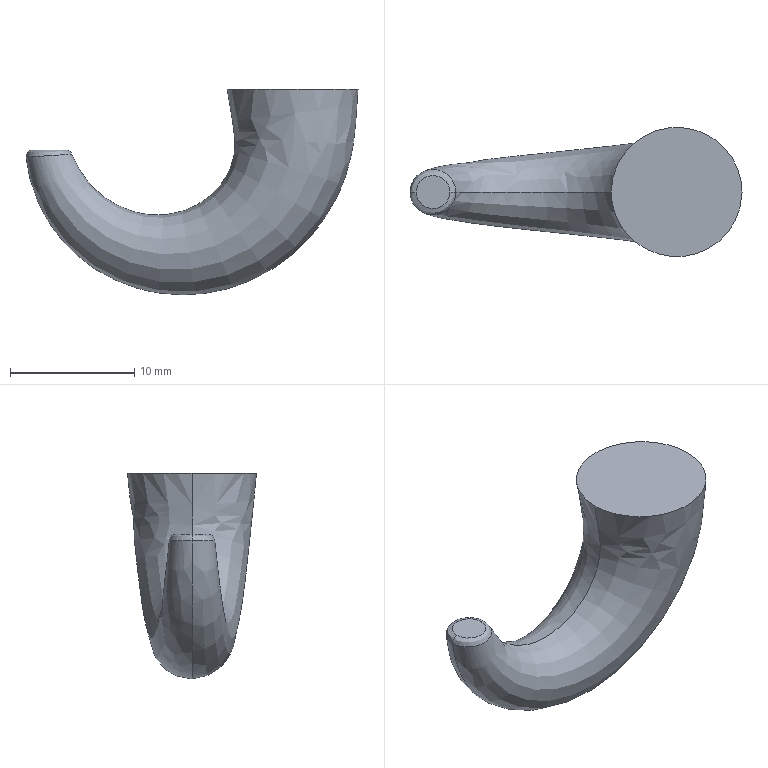Part | STEP file | solid 221 | 1 solid | 6 faces | box 26.698 x 10.392 x 16.548 mm | volume 1362 mm3 | spline 4 | plane 2